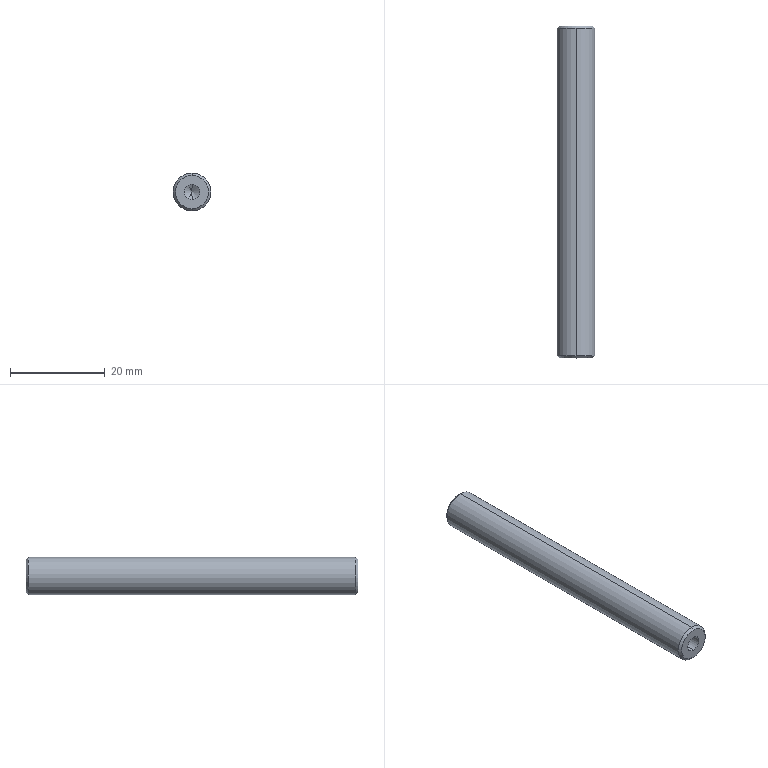Part | SolidWorks | features Chamfer 1, Extrusion 1, HoleWzd 1 | 1 solid | 12 faces | box 8 x 70 x 8 mm | volume 3389 mm3 | cone 6 | cylinder 4 | plane 2 | commonest cylinder face diameters 3.3 x2 8 x2
STEP:
#1=CARTESIAN_POINT('',(0.,14.1,1.65));
#2=VERTEX_POINT('',#1);
#3=CARTESIAN_POINT('',(0.,14.1,-1.65));
#4=VERTEX_POINT('',#3);
#5=CARTESIAN_POINT('',(0.,14.1,0.));
#6=DIRECTION('',(0.,-1.,0.));
#7=DIRECTION('',(0.,0.,-1.));
#8=AXIS2_PLACEMENT_3D('',#5,#6,#7);
#9=CIRCLE('',#8,1.65);
#10=EDGE_CURVE('',#2,#4,#9,.T.);
#11=ORIENTED_EDGE('',*,*,#10,.F.);
#12=CARTESIAN_POINT('',(0.,0.,1.65));
#13=VERTEX_POINT('',#12);
#14=CARTESIAN_POINT('',(0.,0.,1.65));
#15=DIRECTION('',(0.,-1.,0.));
#16=VECTOR('',#15,1000.);
#17=LINE('',#14,#16);
#18=EDGE_CURVE('',#2,#13,#17,.T.);
#19=ORIENTED_EDGE('',*,*,#18,.T.);
#20=CARTESIAN_POINT('',(0.,0.,-1.65));
#21=VERTEX_POINT('',#20);
#22=CARTESIAN_POINT('',(0.,0.,0.));
#23=DIRECTION('',(0.,-1.,0.));
#24=DIRECTION('',(0.,0.,-1.));
#25=AXIS2_PLACEMENT_3D('',#22,#23,#24);
#26=CIRCLE('',#25,1.65);
#27=EDGE_CURVE('',#13,#21,#26,.T.);
#28=ORIENTED_EDGE('',*,*,#27,.T.);
#29=CARTESIAN_POINT('',(0.,0.,-1.65));
#30=DIRECTION('',(0.,-1.,0.));
#31=VECTOR('',#30,1000.);
#32=LINE('',#29,#31);
#33=EDGE_CURVE('',#4,#21,#32,.T.);
#34=ORIENTED_EDGE('',*,*,#33,.F.);
#35=EDGE_LOOP('',(#11,#19,#28,#34));
#36=FACE_OUTER_BOUND('',#35,.T.);
#37=CARTESIAN_POINT('',(0.,0.,0.));
#38=DIRECTION('',(0.,-1.,0.));
#39=DIRECTION('',(0.,0.,-1.));
#40=AXIS2_PLACEMENT_3D('',#37,#38,#39);
#41=CYLINDRICAL_SURFACE('',#40,1.65);
#42=ADVANCED_FACE('',(#36),#41,.F.);
#43=CARTESIAN_POINT('',(0.,15.091,0.));
#44=VERTEX_POINT('',#43);
#45=CARTESIAN_POINT('',(0.,14.1,-1.65));
#46=DIRECTION('',(0.,-0.515,-0.8572));
#47=VECTOR('',#46,1000.);
#48=LINE('',#45,#47);
#49=EDGE_CURVE('',#44,#4,#48,.T.);
#50=ORIENTED_EDGE('',*,*,#49,.F.);
#51=CARTESIAN_POINT('',(0.,14.1,1.65));
#52=DIRECTION('',(0.,-0.515,0.8572));
#53=VECTOR('',#52,1000.);
#54=LINE('',#51,#53);
#55=EDGE_CURVE('',#44,#2,#54,.T.);
#56=ORIENTED_EDGE('',*,*,#55,.T.);
#57=ORIENTED_EDGE('',*,*,#10,.T.);
#58=EDGE_LOOP('',(#50,#56,#57));
#59=FACE_OUTER_BOUND('',#58,.T.);
#60=CARTESIAN_POINT('',(0.,14.1,0.));
#61=DIRECTION('',(0.,-1.,0.));
#62=DIRECTION('',(0.,0.,-1.));
#63=AXIS2_PLACEMENT_3D('',#60,#61,#62);
#64=CONICAL_SURFACE('',#63,1.65,1.03);
#65=ADVANCED_FACE('',(#59),#64,.F.);
#66=CARTESIAN_POINT('',(0.,0.,-3.5));
#67=VERTEX_POINT('',#66);
#68=CARTESIAN_POINT('',(0.,0.,3.5));
#69=VERTEX_POINT('',#68);
#70=CARTESIAN_POINT('',(0.,0.,0.));
#71=DIRECTION('',(0.,-1.,0.));
#72=DIRECTION('',(0.,0.,1.));
#73=AXIS2_PLACEMENT_3D('',#70,#71,#72);
#74=CIRCLE('',#73,3.5);
#75=EDGE_CURVE('',#67,#69,#74,.T.);
#76=ORIENTED_EDGE('',*,*,#75,.F.);
#77=CARTESIAN_POINT('',(0.,0.5,-4.));
#78=VERTEX_POINT('',#77);
#79=CARTESIAN_POINT('',(0.,0.5,-4.));
#80=DIRECTION('',(0.,0.7071,-0.7071));
#81=VECTOR('',#80,1000.);
#82=LINE('',#79,#81);
#83=EDGE_CURVE('',#67,#78,#82,.T.);
#84=ORIENTED_EDGE('',*,*,#83,.T.);
#85=CARTESIAN_POINT('',(0.,0.5,4.));
#86=VERTEX_POINT('',#85);
#87=CARTESIAN_POINT('',(0.,0.5,0.));
#88=DIRECTION('',(0.,1.,0.));
#89=DIRECTION('',(0.,0.,1.));
#90=AXIS2_PLACEMENT_3D('',#87,#88,#89);
#91=CIRCLE('',#90,4.);
#92=EDGE_CURVE('',#86,#78,#91,.T.);
#93=ORIENTED_EDGE('',*,*,#92,.F.);
#94=CARTESIAN_POINT('',(0.,0.5,4.));
#95=DIRECTION('',(0.,0.7071,0.7071));
#96=VECTOR('',#95,1000.);
#97=LINE('',#94,#96);
#98=EDGE_CURVE('',#69,#86,#97,.T.);
#99=ORIENTED_EDGE('',*,*,#98,.F.);
#100=EDGE_LOOP('',(#76,#84,#93,#99));
#101=FACE_OUTER_BOUND('',#100,.T.);
#102=CARTESIAN_POINT('',(0.,0.5,0.));
#103=DIRECTION('',(0.,1.,0.));
#104=DIRECTION('',(0.,0.,1.));
#105=AXIS2_PLACEMENT_3D('',#102,#103,#104);
#106=CONICAL_SURFACE('',#105,4.,0.7854);
#107=ADVANCED_FACE('',(#101),#106,.T.);
#108=CARTESIAN_POINT('',(0.,70.,3.5));
#109=VERTEX_POINT('',#108);
#110=CARTESIAN_POINT('',(0.,70.,-3.5));
#111=VERTEX_POINT('',#110);
#112=CARTESIAN_POINT('',(0.,70.,0.));
#113=DIRECTION('',(0.,1.,0.));
#114=DIRECTION('',(0.,0.,1.));
#115=AXIS2_PLACEMENT_3D('',#112,#113,#114);
#116=CIRCLE('',#115,3.5);
#117=EDGE_CURVE('',#109,#111,#116,.T.);
#118=ORIENTED_EDGE('',*,*,#117,.F.);
#119=CARTESIAN_POINT('',(0.,69.5,4.));
#120=VERTEX_POINT('',#119);
#121=CARTESIAN_POINT('',(0.,70.,3.5));
#122=DIRECTION('',(0.,-0.7071,0.7071));
#123=VECTOR('',#122,1000.);
#124=LINE('',#121,#123);
#125=EDGE_CURVE('',#109,#120,#124,.T.);
#126=ORIENTED_EDGE('',*,*,#125,.T.);
#127=CARTESIAN_POINT('',(0.,69.5,-4.));
#128=VERTEX_POINT('',#127);
#129=CARTESIAN_POINT('',(0.,69.5,0.));
#130=DIRECTION('',(0.,-1.,0.));
#131=DIRECTION('',(0.,0.,1.));
#132=AXIS2_PLACEMENT_3D('',#129,#130,#131);
#133=CIRCLE('',#132,4.);
#134=EDGE_CURVE('',#128,#120,#133,.T.);
#135=ORIENTED_EDGE('',*,*,#134,.F.);
#136=CARTESIAN_POINT('',(0.,70.,-3.5));
#137=DIRECTION('',(0.,-0.7071,-0.7071));
#138=VECTOR('',#137,1000.);
#139=LINE('',#136,#138);
#140=EDGE_CURVE('',#111,#128,#139,.T.);
#141=ORIENTED_EDGE('',*,*,#140,.F.);
#142=EDGE_LOOP('',(#118,#126,#135,#141));
#143=FACE_OUTER_BOUND('',#142,.T.);
#144=CARTESIAN_POINT('',(0.,70.,0.));
#145=DIRECTION('',(0.,-1.,0.));
#146=DIRECTION('',(0.,0.,-1.));
#147=AXIS2_PLACEMENT_3D('',#144,#145,#146);
#148=CONICAL_SURFACE('',#147,3.5,0.7854);
#149=ADVANCED_FACE('',(#143),#148,.T.);
#150=ORIENTED_EDGE('',*,*,#134,.T.);
#151=CARTESIAN_POINT('',(0.,70.,4.));
#152=DIRECTION('',(0.,-1.,0.));
#153=VECTOR('',#152,1000.);
#154=LINE('',#151,#153);
#155=EDGE_CURVE('',#120,#86,#154,.T.);
#156=ORIENTED_EDGE('',*,*,#155,.T.);
#157=ORIENTED_EDGE('',*,*,#92,.T.);
#158=CARTESIAN_POINT('',(0.,70.,-4.));
#159=DIRECTION('',(0.,-1.,0.));
#160=VECTOR('',#159,1000.);
#161=LINE('',#158,#160);
#162=EDGE_CURVE('',#128,#78,#161,.T.);
#163=ORIENTED_EDGE('',*,*,#162,.F.);
#164=EDGE_LOOP('',(#150,#156,#157,#163));
#165=FACE_OUTER_BOUND('',#164,.T.);
#166=CARTESIAN_POINT('',(0.,70.,0.));
#167=DIRECTION('',(0.,-1.,0.));
#168=DIRECTION('',(0.,0.,-1.));
#169=AXIS2_PLACEMENT_3D('',#166,#167,#168);
#170=CYLINDRICAL_SURFACE('',#169,4.);
#171=ADVANCED_FACE('',(#165),#170,.T.);
#172=ORIENTED_EDGE('',*,*,#155,.F.);
#173=CARTESIAN_POINT('',(0.,69.5,0.));
#174=DIRECTION('',(0.,-1.,0.));
#175=DIRECTION('',(0.,0.,1.));
#176=AXIS2_PLACEMENT_3D('',#173,#174,#175);
#177=CIRCLE('',#176,4.);
#178=EDGE_CURVE('',#120,#128,#177,.T.);
#179=ORIENTED_EDGE('',*,*,#178,.T.);
#180=ORIENTED_EDGE('',*,*,#162,.T.);
#181=CARTESIAN_POINT('',(0.,0.5,0.));
#182=DIRECTION('',(0.,1.,0.));
#183=DIRECTION('',(0.,0.,1.));
#184=AXIS2_PLACEMENT_3D('',#181,#182,#183);
#185=CIRCLE('',#184,4.);
#186=EDGE_CURVE('',#78,#86,#185,.T.);
#187=ORIENTED_EDGE('',*,*,#186,.T.);
#188=EDGE_LOOP('',(#172,#179,#180,#187));
#189=FACE_OUTER_BOUND('',#188,.T.);
#190=CARTESIAN_POINT('',(0.,70.,0.));
#191=DIRECTION('',(0.,-1.,0.));
#192=DIRECTION('',(0.,0.,-1.));
#193=AXIS2_PLACEMENT_3D('',#190,#191,#192);
#194=CYLINDRICAL_SURFACE('',#193,4.);
#195=ADVANCED_FACE('',(#189),#194,.T.);
#196=CARTESIAN_POINT('',(0.,70.,0.));
#197=DIRECTION('',(0.,1.,0.));
#198=DIRECTION('',(0.,0.,1.));
#199=AXIS2_PLACEMENT_3D('',#196,#197,#198);
#200=CIRCLE('',#199,3.5);
#201=EDGE_CURVE('',#111,#109,#200,.T.);
#202=ORIENTED_EDGE('',*,*,#201,.T.);
#203=ORIENTED_EDGE('',*,*,#117,.T.);
#204=EDGE_LOOP('',(#202,#203));
#205=FACE_OUTER_BOUND('',#204,.T.);
#206=CARTESIAN_POINT('',(0.,70.,0.));
#207=DIRECTION('',(0.,1.,0.));
#208=DIRECTION('',(0.,0.,1.));
#209=AXIS2_PLACEMENT_3D('',#206,#207,#208);
#210=PLANE('',#209);
#211=ADVANCED_FACE('',(#205),#210,.T.);
#212=CARTESIAN_POINT('',(0.,0.,0.));
#213=DIRECTION('',(0.,-1.,0.));
#214=DIRECTION('',(0.,0.,-1.));
#215=AXIS2_PLACEMENT_3D('',#212,#213,#214);
#216=CIRCLE('',#215,1.65);
#217=EDGE_CURVE('',#21,#13,#216,.T.);
#218=ORIENTED_EDGE('',*,*,#217,.F.);
#219=ORIENTED_EDGE('',*,*,#27,.F.);
#220=EDGE_LOOP('',(#218,#219));
#221=FACE_BOUND('',#220,.T.);
#222=CARTESIAN_POINT('',(0.,0.,0.));
#223=DIRECTION('',(0.,-1.,0.));
#224=DIRECTION('',(0.,0.,1.));
#225=AXIS2_PLACEMENT_3D('',#222,#223,#224);
#226=CIRCLE('',#225,3.5);
#227=EDGE_CURVE('',#69,#67,#226,.T.);
#228=ORIENTED_EDGE('',*,*,#227,.T.);
#229=ORIENTED_EDGE('',*,*,#75,.T.);
#230=EDGE_LOOP('',(#228,#229));
#231=FACE_OUTER_BOUND('',#230,.T.);
#232=CARTESIAN_POINT('',(0.,0.,0.));
#233=DIRECTION('',(0.,1.,0.));
#234=DIRECTION('',(0.,0.,1.));
#235=AXIS2_PLACEMENT_3D('',#232,#233,#234);
#236=PLANE('',#235);
#237=ADVANCED_FACE('',(#221,#231),#236,.F.);
#238=ORIENTED_EDGE('',*,*,#125,.F.);
#239=ORIENTED_EDGE('',*,*,#201,.F.);
#240=ORIENTED_EDGE('',*,*,#140,.T.);
#241=ORIENTED_EDGE('',*,*,#178,.F.);
#242=EDGE_LOOP('',(#238,#239,#240,#241));
#243=FACE_OUTER_BOUND('',#242,.T.);
#244=CARTESIAN_POINT('',(0.,70.,0.));
#245=DIRECTION('',(0.,-1.,0.));
#246=DIRECTION('',(0.,0.,-1.));
#247=AXIS2_PLACEMENT_3D('',#244,#245,#246);
#248=CONICAL_SURFACE('',#247,3.5,0.7854);
#249=ADVANCED_FACE('',(#243),#248,.T.);
#250=ORIENTED_EDGE('',*,*,#83,.F.);
#251=ORIENTED_EDGE('',*,*,#227,.F.);
#252=ORIENTED_EDGE('',*,*,#98,.T.);
#253=ORIENTED_EDGE('',*,*,#186,.F.);
#254=EDGE_LOOP('',(#250,#251,#252,#253));
#255=FACE_OUTER_BOUND('',#254,.T.);
#256=CARTESIAN_POINT('',(0.,0.5,0.));
#257=DIRECTION('',(0.,1.,0.));
#258=DIRECTION('',(0.,0.,1.));
#259=AXIS2_PLACEMENT_3D('',#256,#257,#258);
#260=CONICAL_SURFACE('',#259,4.,0.7854);
#261=ADVANCED_FACE('',(#255),#260,.T.);
#262=ORIENTED_EDGE('',*,*,#55,.F.);
#263=ORIENTED_EDGE('',*,*,#49,.T.);
#264=CARTESIAN_POINT('',(0.,14.1,0.));
#265=DIRECTION('',(0.,-1.,0.));
#266=DIRECTION('',(0.,0.,-1.));
#267=AXIS2_PLACEMENT_3D('',#264,#265,#266);
#268=CIRCLE('',#267,1.65);
#269=EDGE_CURVE('',#4,#2,#268,.T.);
#270=ORIENTED_EDGE('',*,*,#269,.T.);
#271=EDGE_LOOP('',(#262,#263,#270));
#272=FACE_OUTER_BOUND('',#271,.T.);
#273=CARTESIAN_POINT('',(0.,14.1,0.));
#274=DIRECTION('',(0.,-1.,0.));
#275=DIRECTION('',(0.,0.,-1.));
#276=AXIS2_PLACEMENT_3D('',#273,#274,#275);
#277=CONICAL_SURFACE('',#276,1.65,1.03);
#278=ADVANCED_FACE('',(#272),#277,.F.);
#279=ORIENTED_EDGE('',*,*,#18,.F.);
#280=ORIENTED_EDGE('',*,*,#269,.F.);
#281=ORIENTED_EDGE('',*,*,#33,.T.);
#282=ORIENTED_EDGE('',*,*,#217,.T.);
#283=EDGE_LOOP('',(#279,#280,#281,#282));
#284=FACE_OUTER_BOUND('',#283,.T.);
#285=CARTESIAN_POINT('',(0.,0.,0.));
#286=DIRECTION('',(0.,-1.,0.));
#287=DIRECTION('',(0.,0.,-1.));
#288=AXIS2_PLACEMENT_3D('',#285,#286,#287);
#289=CYLINDRICAL_SURFACE('',#288,1.65);
#290=ADVANCED_FACE('',(#284),#289,.F.);
#291=CLOSED_SHELL('',(#42,#65,#107,#149,#171,#195,#211,#237,#249,#261,#278,#290));
#292=MANIFOLD_SOLID_BREP('',#291);
#293=CARTESIAN_POINT('',(0.,0.,0.));
#294=DIRECTION('',(0.,0.,1.));
#295=DIRECTION('',(1.,0.,0.));
#296=AXIS2_PLACEMENT_3D('',#293,#294,#295);
#297=(LENGTH_UNIT()NAMED_UNIT(*)SI_UNIT(.MILLI.,.METRE.));
#298=UNCERTAINTY_MEASURE_WITH_UNIT(LENGTH_MEASURE(0.00001),#297,'','');
#299=(NAMED_UNIT(*)PLANE_ANGLE_UNIT()SI_UNIT($,.RADIAN.));
#300=(NAMED_UNIT(*)SI_UNIT($,.STERADIAN.)SOLID_ANGLE_UNIT());
#301=(GEOMETRIC_REPRESENTATION_CONTEXT(3)GLOBAL_UNCERTAINTY_ASSIGNED_CONTEXT((#298))GLOBAL_UNIT_ASSIGNED_CONTEXT((#297,#299,#300))REPRESENTATION_CONTEXT('',''));
#302=ADVANCED_BREP_SHAPE_REPRESENTATION('',(#292,#296),#301);